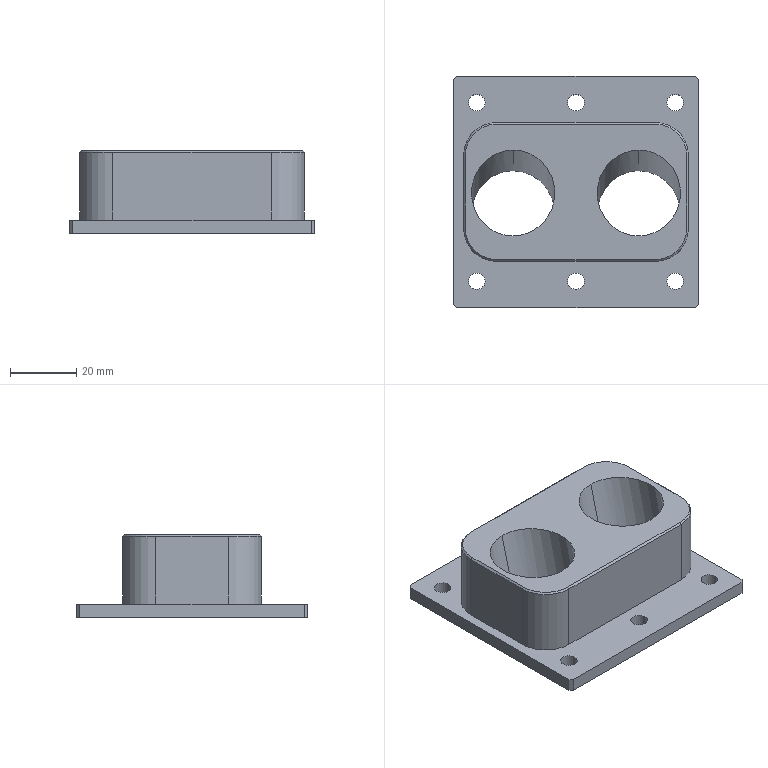Part | SolidWorks | features Chamfer 2, Extrusion 1, ICE 1, MirrorPattern 1, SweepCut 1 | 1 solid | 43 faces | box 74 x 70 x 25 mm | volume 52689 mm3 | cylinder 20 | plane 19 | cone 4 | commonest cylinder face diameters 5 x12 20 x4 25.2 x4
STEP:
#1=CARTESIAN_POINT('',(-19.,-19.566,0.));
#2=VERTEX_POINT('',#1);
#3=CARTESIAN_POINT('',(-19.,6.406,0.));
#4=VERTEX_POINT('',#3);
#5=CARTESIAN_POINT('',(-19.,-19.566,0.));
#6=CARTESIAN_POINT('',(-44.2,-19.566,0.));
#7=CARTESIAN_POINT('',(-44.2,6.406,0.));
#8=CARTESIAN_POINT('',(-19.,6.406,0.));
#9=(BOUNDED_CURVE()B_SPLINE_CURVE(3,(#5,#6,#7,#8),.UNSPECIFIED.,.F.,.F.)B_SPLINE_CURVE_WITH_KNOTS((4,4),(3.142,6.283),.UNSPECIFIED.)CURVE()GEOMETRIC_REPRESENTATION_ITEM()RATIONAL_B_SPLINE_CURVE((1.,0.3333,0.3333,1.))REPRESENTATION_ITEM(''));
#10=EDGE_CURVE('',#2,#4,#9,.T.);
#11=ORIENTED_EDGE('',*,*,#10,.T.);
#12=CARTESIAN_POINT('',(-19.,12.639,25.));
#13=VERTEX_POINT('',#12);
#14=CARTESIAN_POINT('',(-19.,4.636,-7.097));
#15=DIRECTION('',(0.,0.2419,0.9703));
#16=VECTOR('',#15,1000.);
#17=LINE('',#14,#16);
#18=EDGE_CURVE('',#4,#13,#17,.T.);
#19=ORIENTED_EDGE('',*,*,#18,.T.);
#20=CARTESIAN_POINT('',(-19.,-13.333,25.));
#21=VERTEX_POINT('',#20);
#22=CARTESIAN_POINT('',(-19.,12.639,25.));
#23=CARTESIAN_POINT('',(-44.2,12.639,25.));
#24=CARTESIAN_POINT('',(-44.2,-13.333,25.));
#25=CARTESIAN_POINT('',(-19.,-13.333,25.));
#26=(BOUNDED_CURVE()B_SPLINE_CURVE(3,(#22,#23,#24,#25),.UNSPECIFIED.,.F.,.F.)B_SPLINE_CURVE_WITH_KNOTS((4,4),(0.,3.142),.UNSPECIFIED.)CURVE()GEOMETRIC_REPRESENTATION_ITEM()RATIONAL_B_SPLINE_CURVE((1.,0.3333,0.3333,1.))REPRESENTATION_ITEM(''));
#27=EDGE_CURVE('',#13,#21,#26,.T.);
#28=ORIENTED_EDGE('',*,*,#27,.T.);
#29=CARTESIAN_POINT('',(-19.,-19.815,-1.001));
#30=DIRECTION('',(0.,0.2419,0.9703));
#31=VECTOR('',#30,1000.);
#32=LINE('',#29,#31);
#33=EDGE_CURVE('',#2,#21,#32,.T.);
#34=ORIENTED_EDGE('',*,*,#33,.F.);
#35=EDGE_LOOP('',(#11,#19,#28,#34));
#36=FACE_OUTER_BOUND('',#35,.T.);
#37=CARTESIAN_POINT('',(-19.,-7.59,-4.049));
#38=DIRECTION('',(0.,0.2419,0.9703));
#39=DIRECTION('',(0.,-0.9703,0.2419));
#40=AXIS2_PLACEMENT_3D('',#37,#38,#39);
#41=CYLINDRICAL_SURFACE('',#40,12.6);
#42=ADVANCED_FACE('',(#36),#41,.F.);
#43=CARTESIAN_POINT('',(19.,-19.566,0.));
#44=VERTEX_POINT('',#43);
#45=CARTESIAN_POINT('',(19.,6.406,0.));
#46=VERTEX_POINT('',#45);
#47=CARTESIAN_POINT('',(19.,-19.566,0.));
#48=CARTESIAN_POINT('',(-6.2,-19.566,0.));
#49=CARTESIAN_POINT('',(-6.2,6.406,0.));
#50=CARTESIAN_POINT('',(19.,6.406,0.));
#51=(BOUNDED_CURVE()B_SPLINE_CURVE(3,(#47,#48,#49,#50),.UNSPECIFIED.,.F.,.F.)B_SPLINE_CURVE_WITH_KNOTS((4,4),(3.142,6.283),.UNSPECIFIED.)CURVE()GEOMETRIC_REPRESENTATION_ITEM()RATIONAL_B_SPLINE_CURVE((1.,0.3333,0.3333,1.))REPRESENTATION_ITEM(''));
#52=EDGE_CURVE('',#44,#46,#51,.T.);
#53=ORIENTED_EDGE('',*,*,#52,.T.);
#54=CARTESIAN_POINT('',(19.,12.639,25.));
#55=VERTEX_POINT('',#54);
#56=CARTESIAN_POINT('',(19.,4.636,-7.097));
#57=DIRECTION('',(0.,0.2419,0.9703));
#58=VECTOR('',#57,1000.);
#59=LINE('',#56,#58);
#60=EDGE_CURVE('',#46,#55,#59,.T.);
#61=ORIENTED_EDGE('',*,*,#60,.T.);
#62=CARTESIAN_POINT('',(19.,-13.333,25.));
#63=VERTEX_POINT('',#62);
#64=CARTESIAN_POINT('',(19.,12.639,25.));
#65=CARTESIAN_POINT('',(-6.2,12.639,25.));
#66=CARTESIAN_POINT('',(-6.2,-13.333,25.));
#67=CARTESIAN_POINT('',(19.,-13.333,25.));
#68=(BOUNDED_CURVE()B_SPLINE_CURVE(3,(#64,#65,#66,#67),.UNSPECIFIED.,.F.,.F.)B_SPLINE_CURVE_WITH_KNOTS((4,4),(0.,3.142),.UNSPECIFIED.)CURVE()GEOMETRIC_REPRESENTATION_ITEM()RATIONAL_B_SPLINE_CURVE((1.,0.3333,0.3333,1.))REPRESENTATION_ITEM(''));
#69=EDGE_CURVE('',#55,#63,#68,.T.);
#70=ORIENTED_EDGE('',*,*,#69,.T.);
#71=CARTESIAN_POINT('',(19.,-19.815,-1.001));
#72=DIRECTION('',(0.,0.2419,0.9703));
#73=VECTOR('',#72,1000.);
#74=LINE('',#71,#73);
#75=EDGE_CURVE('',#44,#63,#74,.T.);
#76=ORIENTED_EDGE('',*,*,#75,.F.);
#77=EDGE_LOOP('',(#53,#61,#70,#76));
#78=FACE_OUTER_BOUND('',#77,.T.);
#79=CARTESIAN_POINT('',(19.,-7.59,-4.049));
#80=DIRECTION('',(0.,0.2419,0.9703));
#81=DIRECTION('',(0.,-0.9703,0.2419));
#82=AXIS2_PLACEMENT_3D('',#79,#80,#81);
#83=CYLINDRICAL_SURFACE('',#82,12.6);
#84=ADVANCED_FACE('',(#78),#83,.F.);
#85=CARTESIAN_POINT('',(-32.5,-27.,4.));
#86=VERTEX_POINT('',#85);
#87=CARTESIAN_POINT('',(-27.5,-27.,4.));
#88=VERTEX_POINT('',#87);
#89=CARTESIAN_POINT('',(-30.,-27.,4.));
#90=DIRECTION('',(0.,0.,1.));
#91=DIRECTION('',(1.,0.,0.));
#92=AXIS2_PLACEMENT_3D('',#89,#90,#91);
#93=CIRCLE('',#92,2.5);
#94=EDGE_CURVE('',#86,#88,#93,.T.);
#95=ORIENTED_EDGE('',*,*,#94,.T.);
#96=CARTESIAN_POINT('',(-27.5,-27.,0.));
#97=VERTEX_POINT('',#96);
#98=CARTESIAN_POINT('',(-27.5,-27.,4.));
#99=DIRECTION('',(0.,0.,-1.));
#100=VECTOR('',#99,1000.);
#101=LINE('',#98,#100);
#102=EDGE_CURVE('',#88,#97,#101,.T.);
#103=ORIENTED_EDGE('',*,*,#102,.T.);
#104=CARTESIAN_POINT('',(-32.5,-27.,0.));
#105=VERTEX_POINT('',#104);
#106=CARTESIAN_POINT('',(-30.,-27.,0.));
#107=DIRECTION('',(0.,0.,1.));
#108=DIRECTION('',(1.,0.,0.));
#109=AXIS2_PLACEMENT_3D('',#106,#107,#108);
#110=CIRCLE('',#109,2.5);
#111=EDGE_CURVE('',#105,#97,#110,.T.);
#112=ORIENTED_EDGE('',*,*,#111,.F.);
#113=CARTESIAN_POINT('',(-32.5,-27.,4.));
#114=DIRECTION('',(0.,0.,-1.));
#115=VECTOR('',#114,1000.);
#116=LINE('',#113,#115);
#117=EDGE_CURVE('',#86,#105,#116,.T.);
#118=ORIENTED_EDGE('',*,*,#117,.F.);
#119=EDGE_LOOP('',(#95,#103,#112,#118));
#120=FACE_OUTER_BOUND('',#119,.T.);
#121=CARTESIAN_POINT('',(-30.,-27.,4.));
#122=DIRECTION('',(0.,0.,-1.));
#123=DIRECTION('',(-1.,0.,0.));
#124=AXIS2_PLACEMENT_3D('',#121,#122,#123);
#125=CYLINDRICAL_SURFACE('',#124,2.5);
#126=ADVANCED_FACE('',(#120),#125,.F.);
#127=CARTESIAN_POINT('',(-2.5,-27.,4.));
#128=VERTEX_POINT('',#127);
#129=CARTESIAN_POINT('',(2.5,-27.,4.));
#130=VERTEX_POINT('',#129);
#131=CARTESIAN_POINT('',(0.,-27.,4.));
#132=DIRECTION('',(0.,0.,1.));
#133=DIRECTION('',(1.,0.,0.));
#134=AXIS2_PLACEMENT_3D('',#131,#132,#133);
#135=CIRCLE('',#134,2.5);
#136=EDGE_CURVE('',#128,#130,#135,.T.);
#137=ORIENTED_EDGE('',*,*,#136,.T.);
#138=CARTESIAN_POINT('',(2.5,-27.,0.));
#139=VERTEX_POINT('',#138);
#140=CARTESIAN_POINT('',(2.5,-27.,4.));
#141=DIRECTION('',(0.,0.,-1.));
#142=VECTOR('',#141,1000.);
#143=LINE('',#140,#142);
#144=EDGE_CURVE('',#130,#139,#143,.T.);
#145=ORIENTED_EDGE('',*,*,#144,.T.);
#146=CARTESIAN_POINT('',(-2.5,-27.,0.));
#147=VERTEX_POINT('',#146);
#148=CARTESIAN_POINT('',(0.,-27.,0.));
#149=DIRECTION('',(0.,0.,1.));
#150=DIRECTION('',(1.,0.,0.));
#151=AXIS2_PLACEMENT_3D('',#148,#149,#150);
#152=CIRCLE('',#151,2.5);
#153=EDGE_CURVE('',#147,#139,#152,.T.);
#154=ORIENTED_EDGE('',*,*,#153,.F.);
#155=CARTESIAN_POINT('',(-2.5,-27.,4.));
#156=DIRECTION('',(0.,0.,-1.));
#157=VECTOR('',#156,1000.);
#158=LINE('',#155,#157);
#159=EDGE_CURVE('',#128,#147,#158,.T.);
#160=ORIENTED_EDGE('',*,*,#159,.F.);
#161=EDGE_LOOP('',(#137,#145,#154,#160));
#162=FACE_OUTER_BOUND('',#161,.T.);
#163=CARTESIAN_POINT('',(0.,-27.,4.));
#164=DIRECTION('',(0.,0.,-1.));
#165=DIRECTION('',(-1.,0.,0.));
#166=AXIS2_PLACEMENT_3D('',#163,#164,#165);
#167=CYLINDRICAL_SURFACE('',#166,2.5);
#168=ADVANCED_FACE('',(#162),#167,.F.);
#169=CARTESIAN_POINT('',(27.5,-27.,4.));
#170=VERTEX_POINT('',#169);
#171=CARTESIAN_POINT('',(32.5,-27.,4.));
#172=VERTEX_POINT('',#171);
#173=CARTESIAN_POINT('',(30.,-27.,4.));
#174=DIRECTION('',(0.,0.,1.));
#175=DIRECTION('',(1.,0.,0.));
#176=AXIS2_PLACEMENT_3D('',#173,#174,#175);
#177=CIRCLE('',#176,2.5);
#178=EDGE_CURVE('',#170,#172,#177,.T.);
#179=ORIENTED_EDGE('',*,*,#178,.T.);
#180=CARTESIAN_POINT('',(32.5,-27.,0.));
#181=VERTEX_POINT('',#180);
#182=CARTESIAN_POINT('',(32.5,-27.,4.));
#183=DIRECTION('',(0.,0.,-1.));
#184=VECTOR('',#183,1000.);
#185=LINE('',#182,#184);
#186=EDGE_CURVE('',#172,#181,#185,.T.);
#187=ORIENTED_EDGE('',*,*,#186,.T.);
#188=CARTESIAN_POINT('',(27.5,-27.,0.));
#189=VERTEX_POINT('',#188);
#190=CARTESIAN_POINT('',(30.,-27.,0.));
#191=DIRECTION('',(0.,0.,1.));
#192=DIRECTION('',(1.,0.,0.));
#193=AXIS2_PLACEMENT_3D('',#190,#191,#192);
#194=CIRCLE('',#193,2.5);
#195=EDGE_CURVE('',#189,#181,#194,.T.);
#196=ORIENTED_EDGE('',*,*,#195,.F.);
#197=CARTESIAN_POINT('',(27.5,-27.,4.));
#198=DIRECTION('',(0.,0.,-1.));
#199=VECTOR('',#198,1000.);
#200=LINE('',#197,#199);
#201=EDGE_CURVE('',#170,#189,#200,.T.);
#202=ORIENTED_EDGE('',*,*,#201,.F.);
#203=EDGE_LOOP('',(#179,#187,#196,#202));
#204=FACE_OUTER_BOUND('',#203,.T.);
#205=CARTESIAN_POINT('',(30.,-27.,4.));
#206=DIRECTION('',(0.,0.,-1.));
#207=DIRECTION('',(-1.,0.,0.));
#208=AXIS2_PLACEMENT_3D('',#205,#206,#207);
#209=CYLINDRICAL_SURFACE('',#208,2.5);
#210=ADVANCED_FACE('',(#204),#209,.F.);
#211=CARTESIAN_POINT('',(27.5,27.,4.));
#212=VERTEX_POINT('',#211);
#213=CARTESIAN_POINT('',(32.5,27.,4.));
#214=VERTEX_POINT('',#213);
#215=CARTESIAN_POINT('',(30.,27.,4.));
#216=DIRECTION('',(0.,0.,1.));
#217=DIRECTION('',(1.,0.,0.));
#218=AXIS2_PLACEMENT_3D('',#215,#216,#217);
#219=CIRCLE('',#218,2.5);
#220=EDGE_CURVE('',#212,#214,#219,.T.);
#221=ORIENTED_EDGE('',*,*,#220,.T.);
#222=CARTESIAN_POINT('',(32.5,27.,0.));
#223=VERTEX_POINT('',#222);
#224=CARTESIAN_POINT('',(32.5,27.,4.));
#225=DIRECTION('',(0.,0.,-1.));
#226=VECTOR('',#225,1000.);
#227=LINE('',#224,#226);
#228=EDGE_CURVE('',#214,#223,#227,.T.);
#229=ORIENTED_EDGE('',*,*,#228,.T.);
#230=CARTESIAN_POINT('',(27.5,27.,0.));
#231=VERTEX_POINT('',#230);
#232=CARTESIAN_POINT('',(30.,27.,0.));
#233=DIRECTION('',(0.,0.,1.));
#234=DIRECTION('',(1.,0.,0.));
#235=AXIS2_PLACEMENT_3D('',#232,#233,#234);
#236=CIRCLE('',#235,2.5);
#237=EDGE_CURVE('',#231,#223,#236,.T.);
#238=ORIENTED_EDGE('',*,*,#237,.F.);
#239=CARTESIAN_POINT('',(27.5,27.,4.));
#240=DIRECTION('',(0.,0.,-1.));
#241=VECTOR('',#240,1000.);
#242=LINE('',#239,#241);
#243=EDGE_CURVE('',#212,#231,#242,.T.);
#244=ORIENTED_EDGE('',*,*,#243,.F.);
#245=EDGE_LOOP('',(#221,#229,#238,#244));
#246=FACE_OUTER_BOUND('',#245,.T.);
#247=CARTESIAN_POINT('',(30.,27.,4.));
#248=DIRECTION('',(0.,0.,-1.));
#249=DIRECTION('',(-1.,0.,0.));
#250=AXIS2_PLACEMENT_3D('',#247,#248,#249);
#251=CYLINDRICAL_SURFACE('',#250,2.5);
#252=ADVANCED_FACE('',(#246),#251,.F.);
#253=CARTESIAN_POINT('',(-2.5,27.,4.));
#254=VERTEX_POINT('',#253);
#255=CARTESIAN_POINT('',(2.5,27.,4.));
#256=VERTEX_POINT('',#255);
#257=CARTESIAN_POINT('',(0.,27.,4.));
#258=DIRECTION('',(0.,0.,1.));
#259=DIRECTION('',(1.,0.,0.));
#260=AXIS2_PLACEMENT_3D('',#257,#258,#259);
#261=CIRCLE('',#260,2.5);
#262=EDGE_CURVE('',#254,#256,#261,.T.);
#263=ORIENTED_EDGE('',*,*,#262,.T.);
#264=CARTESIAN_POINT('',(2.5,27.,0.));
#265=VERTEX_POINT('',#264);
#266=CARTESIAN_POINT('',(2.5,27.,4.));
#267=DIRECTION('',(0.,0.,-1.));
#268=VECTOR('',#267,1000.);
#269=LINE('',#266,#268);
#270=EDGE_CURVE('',#256,#265,#269,.T.);
#271=ORIENTED_EDGE('',*,*,#270,.T.);
#272=CARTESIAN_POINT('',(-2.5,27.,0.));
#273=VERTEX_POINT('',#272);
#274=CARTESIAN_POINT('',(0.,27.,0.));
#275=DIRECTION('',(0.,0.,1.));
#276=DIRECTION('',(1.,0.,0.));
#277=AXIS2_PLACEMENT_3D('',#274,#275,#276);
#278=CIRCLE('',#277,2.5);
#279=EDGE_CURVE('',#273,#265,#278,.T.);
#280=ORIENTED_EDGE('',*,*,#279,.F.);
#281=CARTESIAN_POINT('',(-2.5,27.,4.));
#282=DIRECTION('',(0.,0.,-1.));
#283=VECTOR('',#282,1000.);
#284=LINE('',#281,#283);
#285=EDGE_CURVE('',#254,#273,#284,.T.);
#286=ORIENTED_EDGE('',*,*,#285,.F.);
#287=EDGE_LOOP('',(#263,#271,#280,#286));
#288=FACE_OUTER_BOUND('',#287,.T.);
#289=CARTESIAN_POINT('',(0.,27.,4.));
#290=DIRECTION('',(0.,0.,-1.));
#291=DIRECTION('',(-1.,0.,0.));
#292=AXIS2_PLACEMENT_3D('',#289,#290,#291);
#293=CYLINDRICAL_SURFACE('',#292,2.5);
#294=ADVANCED_FACE('',(#288),#293,.F.);
#295=CARTESIAN_POINT('',(-32.5,27.,4.));
#296=VERTEX_POINT('',#295);
#297=CARTESIAN_POINT('',(-27.5,27.,4.));
#298=VERTEX_POINT('',#297);
#299=CARTESIAN_POINT('',(-30.,27.,4.));
#300=DIRECTION('',(0.,0.,1.));
#301=DIRECTION('',(1.,0.,0.));
#302=AXIS2_PLACEMENT_3D('',#299,#300,#301);
#303=CIRCLE('',#302,2.5);
#304=EDGE_CURVE('',#296,#298,#303,.T.);
#305=ORIENTED_EDGE('',*,*,#304,.T.);
#306=CARTESIAN_POINT('',(-27.5,27.,0.));
#307=VERTEX_POINT('',#306);
#308=CARTESIAN_POINT('',(-27.5,27.,4.));
#309=DIRECTION('',(0.,0.,-1.));
#310=VECTOR('',#309,1000.);
#311=LINE('',#308,#310);
#312=EDGE_CURVE('',#298,#307,#311,.T.);
#313=ORIENTED_EDGE('',*,*,#312,.T.);
#314=CARTESIAN_POINT('',(-32.5,27.,0.));
#315=VERTEX_POINT('',#314);
#316=CARTESIAN_POINT('',(-30.,27.,0.));
#317=DIRECTION('',(0.,0.,1.));
#318=DIRECTION('',(1.,0.,0.));
#319=AXIS2_PLACEMENT_3D('',#316,#317,#318);
#320=CIRCLE('',#319,2.5);
#321=EDGE_CURVE('',#315,#307,#320,.T.);
#322=ORIENTED_EDGE('',*,*,#321,.F.);
#323=CARTESIAN_POINT('',(-32.5,27.,4.));
#324=DIRECTION('',(0.,0.,-1.));
#325=VECTOR('',#324,1000.);
#326=LINE('',#323,#325);
#327=EDGE_CURVE('',#296,#315,#326,.T.);
#328=ORIENTED_EDGE('',*,*,#327,.F.);
#329=EDGE_LOOP('',(#305,#313,#322,#328));
#330=FACE_OUTER_BOUND('',#329,.T.);
#331=CARTESIAN_POINT('',(-30.,27.,4.));
#332=DIRECTION('',(0.,0.,-1.));
#333=DIRECTION('',(-1.,0.,0.));
#334=AXIS2_PLACEMENT_3D('',#331,#332,#333);
#335=CYLINDRICAL_SURFACE('',#334,2.5);
#336=ADVANCED_FACE('',(#330),#335,.F.);
#337=ORIENTED_EDGE('',*,*,#94,.F.);
#338=CARTESIAN_POINT('',(-30.,-27.,4.));
#339=DIRECTION('',(0.,0.,1.));
#340=DIRECTION('',(1.,0.,0.));
#341=AXIS2_PLACEMENT_3D('',#338,#339,#340);
#342=CIRCLE('',#341,2.5);
#343=EDGE_CURVE('',#88,#86,#342,.T.);
#344=ORIENTED_EDGE('',*,*,#343,.F.);
#345=EDGE_LOOP('',(#337,#344));
#346=FACE_BOUND('',#345,.T.);
#347=ORIENTED_EDGE('',*,*,#136,.F.);
#348=CARTESIAN_POINT('',(0.,-27.,4.));
#349=DIRECTION('',(0.,0.,1.));
#350=DIRECTION('',(1.,0.,0.));
#351=AXIS2_PLACEMENT_3D('',#348,#349,#350);
#352=CIRCLE('',#351,2.5);
#353=EDGE_CURVE('',#130,#128,#352,.T.);
#354=ORIENTED_EDGE('',*,*,#353,.F.);
#355=EDGE_LOOP('',(#347,#354));
#356=FACE_BOUND('',#355,.T.);
#357=ORIENTED_EDGE('',*,*,#178,.F.);
#358=CARTESIAN_POINT('',(30.,-27.,4.));
#359=DIRECTION('',(0.,0.,1.));
#360=DIRECTION('',(1.,0.,0.));
#361=AXIS2_PLACEMENT_3D('',#358,#359,#360);
#362=CIRCLE('',#361,2.5);
#363=EDGE_CURVE('',#172,#170,#362,.T.);
#364=ORIENTED_EDGE('',*,*,#363,.F.);
#365=EDGE_LOOP('',(#357,#364));
#366=FACE_BOUND('',#365,.T.);
#367=ORIENTED_EDGE('',*,*,#220,.F.);
#368=CARTESIAN_POINT('',(30.,27.,4.));
#369=DIRECTION('',(0.,0.,1.));
#370=DIRECTION('',(1.,0.,0.));
#371=AXIS2_PLACEMENT_3D('',#368,#369,#370);
#372=CIRCLE('',#371,2.5);
#373=EDGE_CURVE('',#214,#212,#372,.T.);
#374=ORIENTED_EDGE('',*,*,#373,.F.);
#375=EDGE_LOOP('',(#367,#374));
#376=FACE_BOUND('',#375,.T.);
#377=ORIENTED_EDGE('',*,*,#262,.F.);
#378=CARTESIAN_POINT('',(0.,27.,4.));
#379=DIRECTION('',(0.,0.,1.));
#380=DIRECTION('',(1.,0.,0.));
#381=AXIS2_PLACEMENT_3D('',#378,#379,#380);
#382=CIRCLE('',#381,2.5);
#383=EDGE_CURVE('',#256,#254,#382,.T.);
#384=ORIENTED_EDGE('',*,*,#383,.F.);
#385=EDGE_LOOP('',(#377,#384));
#386=FACE_BOUND('',#385,.T.);
#387=ORIENTED_EDGE('',*,*,#304,.F.);
#388=CARTESIAN_POINT('',(-30.,27.,4.));
#389=DIRECTION('',(0.,0.,1.));
#390=DIRECTION('',(1.,0.,0.));
#391=AXIS2_PLACEMENT_3D('',#388,#389,#390);
#392=CIRCLE('',#391,2.5);
#393=EDGE_CURVE('',#298,#296,#392,.T.);
#394=ORIENTED_EDGE('',*,*,#393,.F.);
#395=EDGE_LOOP('',(#387,#394));
#396=FACE_BOUND('',#395,.T.);
#397=CARTESIAN_POINT('',(-36.,-35.,4.));
#398=VERTEX_POINT('',#397);
#399=CARTESIAN_POINT('',(36.,-35.,4.));
#400=VERTEX_POINT('',#399);
#401=CARTESIAN_POINT('',(0.,-35.,4.));
#402=DIRECTION('',(1.,0.,0.));
#403=VECTOR('',#402,1000.);
#404=LINE('',#401,#403);
#405=EDGE_CURVE('',#398,#400,#404,.T.);
#406=ORIENTED_EDGE('',*,*,#405,.T.);
#407=CARTESIAN_POINT('',(37.,-34.,4.));
#408=VERTEX_POINT('',#407);
#409=CARTESIAN_POINT('',(35.5,-35.5,4.));
#410=DIRECTION('',(0.7071,0.7071,0.));
#411=VECTOR('',#410,1000.);
#412=LINE('',#409,#411);
#413=EDGE_CURVE('',#400,#408,#412,.T.);
#414=ORIENTED_EDGE('',*,*,#413,.T.);
#415=CARTESIAN_POINT('',(37.,34.,4.));
#416=VERTEX_POINT('',#415);
#417=CARTESIAN_POINT('',(37.,0.,4.));
#418=DIRECTION('',(0.,1.,0.));
#419=VECTOR('',#418,1000.);
#420=LINE('',#417,#419);
#421=EDGE_CURVE('',#408,#416,#420,.T.);
#422=ORIENTED_EDGE('',*,*,#421,.T.);
#423=CARTESIAN_POINT('',(36.,35.,4.));
#424=VERTEX_POINT('',#423);
#425=CARTESIAN_POINT('',(35.5,35.5,4.));
#426=DIRECTION('',(-0.7071,0.7071,0.));
#427=VECTOR('',#426,1000.);
#428=LINE('',#425,#427);
#429=EDGE_CURVE('',#416,#424,#428,.T.);
#430=ORIENTED_EDGE('',*,*,#429,.T.);
#431=CARTESIAN_POINT('',(-36.,35.,4.));
#432=VERTEX_POINT('',#431);
#433=CARTESIAN_POINT('',(0.,35.,4.));
#434=DIRECTION('',(1.,0.,0.));
#435=VECTOR('',#434,1000.);
#436=LINE('',#433,#435);
#437=EDGE_CURVE('',#432,#424,#436,.T.);
#438=ORIENTED_EDGE('',*,*,#437,.F.);
#439=CARTESIAN_POINT('',(-37.,34.,4.));
#440=VERTEX_POINT('',#439);
#441=CARTESIAN_POINT('',(-35.5,35.5,4.));
#442=DIRECTION('',(-0.7071,-0.7071,0.));
#443=VECTOR('',#442,1000.);
#444=LINE('',#441,#443);
#445=EDGE_CURVE('',#432,#440,#444,.T.);
#446=ORIENTED_EDGE('',*,*,#445,.T.);
#447=CARTESIAN_POINT('',(-37.,-34.,4.));
#448=VERTEX_POINT('',#447);
#449=CARTESIAN_POINT('',(-37.,0.,4.));
#450=DIRECTION('',(0.,1.,0.));
#451=VECTOR('',#450,1000.);
#452=LINE('',#449,#451);
#453=EDGE_CURVE('',#448,#440,#452,.T.);
#454=ORIENTED_EDGE('',*,*,#453,.F.);
#455=CARTESIAN_POINT('',(-35.5,-35.5,4.));
#456=DIRECTION('',(0.7071,-0.7071,0.));
#457=VECTOR('',#456,1000.);
#458=LINE('',#455,#457);
#459=EDGE_CURVE('',#448,#398,#458,.T.);
#460=ORIENTED_EDGE('',*,*,#459,.T.);
#461=EDGE_LOOP('',(#406,#414,#422,#430,#438,#446,#454,#460));
#462=FACE_OUTER_BOUND('',#461,.T.);
#463=CARTESIAN_POINT('',(24.,21.,4.));
#464=VERTEX_POINT('',#463);
#465=CARTESIAN_POINT('',(-24.,21.,4.));
#466=VERTEX_POINT('',#465);
#467=CARTESIAN_POINT('',(-24.,21.,4.));
#468=DIRECTION('',(-1.,0.,0.));
#469=VECTOR('',#468,1000.);
#470=LINE('',#467,#469);
#471=EDGE_CURVE('',#464,#466,#470,.T.);
#472=ORIENTED_EDGE('',*,*,#471,.F.);
#473=CARTESIAN_POINT('',(34.,11.,4.));
#474=VERTEX_POINT('',#473);
#475=CARTESIAN_POINT('',(24.,11.,4.));
#476=DIRECTION('',(0.,0.,1.));
#477=DIRECTION('',(-1.,0.,0.));
#478=AXIS2_PLACEMENT_3D('',#475,#476,#477);
#479=CIRCLE('',#478,10.);
#480=EDGE_CURVE('',#474,#464,#479,.T.);
#481=ORIENTED_EDGE('',*,*,#480,.F.);
#482=CARTESIAN_POINT('',(34.,-11.,4.));
#483=VERTEX_POINT('',#482);
#484=CARTESIAN_POINT('',(34.,-11.,4.));
#485=DIRECTION('',(0.,1.,0.));
#486=VECTOR('',#485,1000.);
#487=LINE('',#484,#486);
#488=EDGE_CURVE('',#483,#474,#487,.T.);
#489=ORIENTED_EDGE('',*,*,#488,.F.);
#490=CARTESIAN_POINT('',(24.,-21.,4.));
#491=VERTEX_POINT('',#490);
#492=CARTESIAN_POINT('',(24.,-11.,4.));
#493=DIRECTION('',(0.,0.,1.));
#494=DIRECTION('',(-1.,0.,0.));
#495=AXIS2_PLACEMENT_3D('',#492,#493,#494);
#496=CIRCLE('',#495,10.);
#497=EDGE_CURVE('',#491,#483,#496,.T.);
#498=ORIENTED_EDGE('',*,*,#497,.F.);
#499=CARTESIAN_POINT('',(-24.,-21.,4.));
#500=VERTEX_POINT('',#499);
#501=CARTESIAN_POINT('',(-24.,-21.,4.));
#502=DIRECTION('',(1.,0.,0.));
#503=VECTOR('',#502,1000.);
#504=LINE('',#501,#503);
#505=EDGE_CURVE('',#500,#491,#504,.T.);
#506=ORIENTED_EDGE('',*,*,#505,.F.);
#507=CARTESIAN_POINT('',(-34.,-11.,4.));
#508=VERTEX_POINT('',#507);
#509=CARTESIAN_POINT('',(-24.,-11.,4.));
#510=DIRECTION('',(0.,0.,1.));
#511=DIRECTION('',(-1.,0.,0.));
#512=AXIS2_PLACEMENT_3D('',#509,#510,#511);
#513=CIRCLE('',#512,10.);
#514=EDGE_CURVE('',#508,#500,#513,.T.);
#515=ORIENTED_EDGE('',*,*,#514,.F.);
#516=CARTESIAN_POINT('',(-34.,11.,4.));
#517=VERTEX_POINT('',#516);
#518=CARTESIAN_POINT('',(-34.,-11.,4.));
#519=DIRECTION('',(0.,-1.,0.));
#520=VECTOR('',#519,1000.);
#521=LINE('',#518,#520);
#522=EDGE_CURVE('',#517,#508,#521,.T.);
#523=ORIENTED_EDGE('',*,*,#522,.F.);
#524=CARTESIAN_POINT('',(-24.,11.,4.));
#525=DIRECTION('',(0.,0.,1.));
#526=DIRECTION('',(-1.,0.,0.));
#527=AXIS2_PLACEMENT_3D('',#524,#525,#526);
#528=CIRCLE('',#527,10.);
#529=EDGE_CURVE('',#466,#517,#528,.T.);
#530=ORIENTED_EDGE('',*,*,#529,.F.);
#531=EDGE_LOOP('',(#472,#481,#489,#498,#506,#515,#523,#530));
#532=FACE_BOUND('',#531,.T.);
#533=CARTESIAN_POINT('',(0.,0.,4.));
#534=DIRECTION('',(0.,0.,1.));
#535=DIRECTION('',(1.,0.,0.));
#536=AXIS2_PLACEMENT_3D('',#533,#534,#535);
#537=PLANE('',#536);
#538=ADVANCED_FACE('',(#346,#356,#366,#376,#386,#396,#462,#532),#537,.T.);
#539=CARTESIAN_POINT('',(-36.,-35.,0.));
#540=VERTEX_POINT('',#539);
#541=CARTESIAN_POINT('',(36.,-35.,0.));
#542=VERTEX_POINT('',#541);
#543=CARTESIAN_POINT('',(0.,-35.,0.));
#544=DIRECTION('',(1.,0.,0.));
#545=VECTOR('',#544,1000.);
#546=LINE('',#543,#545);
#547=EDGE_CURVE('',#540,#542,#546,.T.);
#548=ORIENTED_EDGE('',*,*,#547,.T.);
#549=CARTESIAN_POINT('',(36.,-35.,4.));
#550=DIRECTION('',(0.,0.,1.));
#551=VECTOR('',#550,1000.);
#552=LINE('',#549,#551);
#553=EDGE_CURVE('',#542,#400,#552,.T.);
#554=ORIENTED_EDGE('',*,*,#553,.T.);
#555=ORIENTED_EDGE('',*,*,#405,.F.);
#556=CARTESIAN_POINT('',(-36.,-35.,0.));
#557=DIRECTION('',(0.,0.,-1.));
#558=VECTOR('',#557,1000.);
#559=LINE('',#556,#558);
#560=EDGE_CURVE('',#398,#540,#559,.T.);
#561=ORIENTED_EDGE('',*,*,#560,.T.);
#562=EDGE_LOOP('',(#548,#554,#555,#561));
#563=FACE_OUTER_BOUND('',#562,.T.);
#564=CARTESIAN_POINT('',(0.,-35.,4.));
#565=DIRECTION('',(0.,1.,0.));
#566=DIRECTION('',(0.,0.,1.));
#567=AXIS2_PLACEMENT_3D('',#564,#565,#566);
#568=PLANE('',#567);
#569=ADVANCED_FACE('',(#563),#568,.F.);
#570=ORIENTED_EDGE('',*,*,#421,.F.);
#571=CARTESIAN_POINT('',(37.,-34.,0.));
#572=VERTEX_POINT('',#571);
#573=CARTESIAN_POINT('',(37.,-34.,4.));
#574=DIRECTION('',(0.,0.,-1.));
#575=VECTOR('',#574,1000.);
#576=LINE('',#573,#575);
#577=EDGE_CURVE('',#408,#572,#576,.T.);
#578=ORIENTED_EDGE('',*,*,#577,.T.);
#579=CARTESIAN_POINT('',(37.,34.,0.));
#580=VERTEX_POINT('',#579);
#581=CARTESIAN_POINT('',(37.,0.,0.));
#582=DIRECTION('',(0.,1.,0.));
#583=VECTOR('',#582,1000.);
#584=LINE('',#581,#583);
#585=EDGE_CURVE('',#572,#580,#584,.T.);
#586=ORIENTED_EDGE('',*,*,#585,.T.);
#587=CARTESIAN_POINT('',(37.,34.,4.));
#588=DIRECTION('',(0.,0.,1.));
#589=VECTOR('',#588,1000.);
#590=LINE('',#587,#589);
#591=EDGE_CURVE('',#580,#416,#590,.T.);
#592=ORIENTED_EDGE('',*,*,#591,.T.);
#593=EDGE_LOOP('',(#570,#578,#586,#592));
#594=FACE_OUTER_BOUND('',#593,.T.);
#595=CARTESIAN_POINT('',(37.,0.,4.));
#596=DIRECTION('',(-1.,0.,0.));
#597=DIRECTION('',(0.,0.,1.));
#598=AXIS2_PLACEMENT_3D('',#595,#596,#597);
#599=PLANE('',#598);
#600=ADVANCED_FACE('',(#594),#599,.F.);
#601=ORIENTED_EDGE('',*,*,#437,.T.);
#602=CARTESIAN_POINT('',(36.,35.,0.));
#603=VERTEX_POINT('',#602);
#604=CARTESIAN_POINT('',(36.,35.,0.));
#605=DIRECTION('',(0.,0.,-1.));
#606=VECTOR('',#605,1000.);
#607=LINE('',#604,#606);
#608=EDGE_CURVE('',#424,#603,#607,.T.);
#609=ORIENTED_EDGE('',*,*,#608,.T.);
#610=CARTESIAN_POINT('',(-36.,35.,0.));
#611=VERTEX_POINT('',#610);
#612=CARTESIAN_POINT('',(0.,35.,0.));
#613=DIRECTION('',(1.,0.,0.));
#614=VECTOR('',#613,1000.);
#615=LINE('',#612,#614);
#616=EDGE_CURVE('',#611,#603,#615,.T.);
#617=ORIENTED_EDGE('',*,*,#616,.F.);
#618=CARTESIAN_POINT('',(-36.,35.,4.));
#619=DIRECTION('',(0.,0.,1.));
#620=VECTOR('',#619,1000.);
#621=LINE('',#618,#620);
#622=EDGE_CURVE('',#611,#432,#621,.T.);
#623=ORIENTED_EDGE('',*,*,#622,.T.);
#624=EDGE_LOOP('',(#601,#609,#617,#623));
#625=FACE_OUTER_BOUND('',#624,.T.);
#626=CARTESIAN_POINT('',(0.,35.,4.));
#627=DIRECTION('',(0.,1.,0.));
#628=DIRECTION('',(0.,0.,1.));
#629=AXIS2_PLACEMENT_3D('',#626,#627,#628);
#630=PLANE('',#629);
#631=ADVANCED_FACE('',(#625),#630,.T.);
#632=ORIENTED_EDGE('',*,*,#312,.F.);
#633=ORIENTED_EDGE('',*,*,#393,.T.);
#634=ORIENTED_EDGE('',*,*,#327,.T.);
#635=CARTESIAN_POINT('',(-30.,27.,0.));
#636=DIRECTION('',(0.,0.,1.));
#637=DIRECTION('',(1.,0.,0.));
#638=AXIS2_PLACEMENT_3D('',#635,#636,#637);
#639=CIRCLE('',#638,2.5);
#640=EDGE_CURVE('',#307,#315,#639,.T.);
#641=ORIENTED_EDGE('',*,*,#640,.F.);
#642=EDGE_LOOP('',(#632,#633,#634,#641));
#643=FACE_OUTER_BOUND('',#642,.T.);
#644=CARTESIAN_POINT('',(-30.,27.,4.));
#645=DIRECTION('',(0.,0.,-1.));
#646=DIRECTION('',(-1.,0.,0.));
#647=AXIS2_PLACEMENT_3D('',#644,#645,#646);
#648=CYLINDRICAL_SURFACE('',#647,2.5);
#649=ADVANCED_FACE('',(#643),#648,.F.);
#650=ORIENTED_EDGE('',*,*,#270,.F.);
#651=ORIENTED_EDGE('',*,*,#383,.T.);
#652=ORIENTED_EDGE('',*,*,#285,.T.);
#653=CARTESIAN_POINT('',(0.,27.,0.));
#654=DIRECTION('',(0.,0.,1.));
#655=DIRECTION('',(1.,0.,0.));
#656=AXIS2_PLACEMENT_3D('',#653,#654,#655);
#657=CIRCLE('',#656,2.5);
#658=EDGE_CURVE('',#265,#273,#657,.T.);
#659=ORIENTED_EDGE('',*,*,#658,.F.);
#660=EDGE_LOOP('',(#650,#651,#652,#659));
#661=FACE_OUTER_BOUND('',#660,.T.);
#662=CARTESIAN_POINT('',(0.,27.,4.));
#663=DIRECTION('',(0.,0.,-1.));
#664=DIRECTION('',(-1.,0.,0.));
#665=AXIS2_PLACEMENT_3D('',#662,#663,#664);
#666=CYLINDRICAL_SURFACE('',#665,2.5);
#667=ADVANCED_FACE('',(#661),#666,.F.);
#668=ORIENTED_EDGE('',*,*,#228,.F.);
#669=ORIENTED_EDGE('',*,*,#373,.T.);
#670=ORIENTED_EDGE('',*,*,#243,.T.);
#671=CARTESIAN_POINT('',(30.,27.,0.));
#672=DIRECTION('',(0.,0.,1.));
#673=DIRECTION('',(1.,0.,0.));
#674=AXIS2_PLACEMENT_3D('',#671,#672,#673);
#675=CIRCLE('',#674,2.5);
#676=EDGE_CURVE('',#223,#231,#675,.T.);
#677=ORIENTED_EDGE('',*,*,#676,.F.);
#678=EDGE_LOOP('',(#668,#669,#670,#677));
#679=FACE_OUTER_BOUND('',#678,.T.);
#680=CARTESIAN_POINT('',(30.,27.,4.));
#681=DIRECTION('',(0.,0.,-1.));
#682=DIRECTION('',(-1.,0.,0.));
#683=AXIS2_PLACEMENT_3D('',#680,#681,#682);
#684=CYLINDRICAL_SURFACE('',#683,2.5);
#685=ADVANCED_FACE('',(#679),#684,.F.);
#686=ORIENTED_EDGE('',*,*,#186,.F.);
#687=ORIENTED_EDGE('',*,*,#363,.T.);
#688=ORIENTED_EDGE('',*,*,#201,.T.);
#689=CARTESIAN_POINT('',(30.,-27.,0.));
#690=DIRECTION('',(0.,0.,1.));
#691=DIRECTION('',(1.,0.,0.));
#692=AXIS2_PLACEMENT_3D('',#689,#690,#691);
#693=CIRCLE('',#692,2.5);
#694=EDGE_CURVE('',#181,#189,#693,.T.);
#695=ORIENTED_EDGE('',*,*,#694,.F.);
#696=EDGE_LOOP('',(#686,#687,#688,#695));
#697=FACE_OUTER_BOUND('',#696,.T.);
#698=CARTESIAN_POINT('',(30.,-27.,4.));
#699=DIRECTION('',(0.,0.,-1.));
#700=DIRECTION('',(-1.,0.,0.));
#701=AXIS2_PLACEMENT_3D('',#698,#699,#700);
#702=CYLINDRICAL_SURFACE('',#701,2.5);
#703=ADVANCED_FACE('',(#697),#702,.F.);
#704=ORIENTED_EDGE('',*,*,#144,.F.);
#705=ORIENTED_EDGE('',*,*,#353,.T.);
#706=ORIENTED_EDGE('',*,*,#159,.T.);
#707=CARTESIAN_POINT('',(0.,-27.,0.));
#708=DIRECTION('',(0.,0.,1.));
#709=DIRECTION('',(1.,0.,0.));
#710=AXIS2_PLACEMENT_3D('',#707,#708,#709);
#711=CIRCLE('',#710,2.5);
#712=EDGE_CURVE('',#139,#147,#711,.T.);
#713=ORIENTED_EDGE('',*,*,#712,.F.);
#714=EDGE_LOOP('',(#704,#705,#706,#713));
#715=FACE_OUTER_BOUND('',#714,.T.);
#716=CARTESIAN_POINT('',(0.,-27.,4.));
#717=DIRECTION('',(0.,0.,-1.));
#718=DIRECTION('',(-1.,0.,0.));
#719=AXIS2_PLACEMENT_3D('',#716,#717,#718);
#720=CYLINDRICAL_SURFACE('',#719,2.5);
#721=ADVANCED_FACE('',(#715),#720,.F.);
#722=ORIENTED_EDGE('',*,*,#102,.F.);
#723=ORIENTED_EDGE('',*,*,#343,.T.);
#724=ORIENTED_EDGE('',*,*,#117,.T.);
#725=CARTESIAN_POINT('',(-30.,-27.,0.));
#726=DIRECTION('',(0.,0.,1.));
#727=DIRECTION('',(1.,0.,0.));
#728=AXIS2_PLACEMENT_3D('',#725,#726,#727);
#729=CIRCLE('',#728,2.5);
#730=EDGE_CURVE('',#97,#105,#729,.T.);
#731=ORIENTED_EDGE('',*,*,#730,.F.);
#732=EDGE_LOOP('',(#722,#723,#724,#731));
#733=FACE_OUTER_BOUND('',#732,.T.);
#734=CARTESIAN_POINT('',(-30.,-27.,4.));
#735=DIRECTION('',(0.,0.,-1.));
#736=DIRECTION('',(-1.,0.,0.));
#737=AXIS2_PLACEMENT_3D('',#734,#735,#736);
#738=CYLINDRICAL_SURFACE('',#737,2.5);
#739=ADVANCED_FACE('',(#733),#738,.F.);
#740=CARTESIAN_POINT('',(-37.,-34.,0.));
#741=VERTEX_POINT('',#740);
#742=CARTESIAN_POINT('',(-37.,34.,0.));
#743=VERTEX_POINT('',#742);
#744=CARTESIAN_POINT('',(-37.,0.,0.));
#745=DIRECTION('',(0.,1.,0.));
#746=VECTOR('',#745,1000.);
#747=LINE('',#744,#746);
#748=EDGE_CURVE('',#741,#743,#747,.T.);
#749=ORIENTED_EDGE('',*,*,#748,.F.);
#750=CARTESIAN_POINT('',(-37.,-34.,4.));
#751=DIRECTION('',(0.,0.,1.));
#752=VECTOR('',#751,1000.);
#753=LINE('',#750,#752);
#754=EDGE_CURVE('',#741,#448,#753,.T.);
#755=ORIENTED_EDGE('',*,*,#754,.T.);
#756=ORIENTED_EDGE('',*,*,#453,.T.);
#757=CARTESIAN_POINT('',(-37.,34.,4.));
#758=DIRECTION('',(0.,0.,-1.));
#759=VECTOR('',#758,1000.);
#760=LINE('',#757,#759);
#761=EDGE_CURVE('',#440,#743,#760,.T.);
#762=ORIENTED_EDGE('',*,*,#761,.T.);
#763=EDGE_LOOP('',(#749,#755,#756,#762));
#764=FACE_OUTER_BOUND('',#763,.T.);
#765=CARTESIAN_POINT('',(-37.,0.,4.));
#766=DIRECTION('',(-1.,0.,0.));
#767=DIRECTION('',(0.,0.,1.));
#768=AXIS2_PLACEMENT_3D('',#765,#766,#767);
#769=PLANE('',#768);
#770=ADVANCED_FACE('',(#764),#769,.T.);
#771=ORIENTED_EDGE('',*,*,#10,.F.);
#772=CARTESIAN_POINT('',(-19.,6.406,0.));
#773=CARTESIAN_POINT('',(6.2,6.406,0.));
#774=CARTESIAN_POINT('',(6.2,-19.566,0.));
#775=CARTESIAN_POINT('',(-19.,-19.566,0.));
#776=(BOUNDED_CURVE()B_SPLINE_CURVE(3,(#772,#773,#774,#775),.UNSPECIFIED.,.F.,.F.)B_SPLINE_CURVE_WITH_KNOTS((4,4),(0.,3.142),.UNSPECIFIED.)CURVE()GEOMETRIC_REPRESENTATION_ITEM()RATIONAL_B_SPLINE_CURVE((1.,0.3333,0.3333,1.))REPRESENTATION_ITEM(''));
#777=EDGE_CURVE('',#4,#2,#776,.T.);
#778=ORIENTED_EDGE('',*,*,#777,.F.);
#779=EDGE_LOOP('',(#771,#778));
#780=FACE_BOUND('',#779,.T.);
#781=ORIENTED_EDGE('',*,*,#52,.F.);
#782=CARTESIAN_POINT('',(19.,6.406,0.));
#783=CARTESIAN_POINT('',(44.2,6.406,0.));
#784=CARTESIAN_POINT('',(44.2,-19.566,0.));
#785=CARTESIAN_POINT('',(19.,-19.566,0.));
#786=(BOUNDED_CURVE()B_SPLINE_CURVE(3,(#782,#783,#784,#785),.UNSPECIFIED.,.F.,.F.)B_SPLINE_CURVE_WITH_KNOTS((4,4),(0.,3.142),.UNSPECIFIED.)CURVE()GEOMETRIC_REPRESENTATION_ITEM()RATIONAL_B_SPLINE_CURVE((1.,0.3333,0.3333,1.))REPRESENTATION_ITEM(''));
#787=EDGE_CURVE('',#46,#44,#786,.T.);
#788=ORIENTED_EDGE('',*,*,#787,.F.);
#789=EDGE_LOOP('',(#781,#788));
#790=FACE_BOUND('',#789,.T.);
#791=ORIENTED_EDGE('',*,*,#111,.T.);
#792=ORIENTED_EDGE('',*,*,#730,.T.);
#793=EDGE_LOOP('',(#791,#792));
#794=FACE_BOUND('',#793,.T.);
#795=ORIENTED_EDGE('',*,*,#153,.T.);
#796=ORIENTED_EDGE('',*,*,#712,.T.);
#797=EDGE_LOOP('',(#795,#796));
#798=FACE_BOUND('',#797,.T.);
#799=ORIENTED_EDGE('',*,*,#195,.T.);
#800=ORIENTED_EDGE('',*,*,#694,.T.);
#801=EDGE_LOOP('',(#799,#800));
#802=FACE_BOUND('',#801,.T.);
#803=ORIENTED_EDGE('',*,*,#237,.T.);
#804=ORIENTED_EDGE('',*,*,#676,.T.);
#805=EDGE_LOOP('',(#803,#804));
#806=FACE_BOUND('',#805,.T.);
#807=ORIENTED_EDGE('',*,*,#279,.T.);
#808=ORIENTED_EDGE('',*,*,#658,.T.);
#809=EDGE_LOOP('',(#807,#808));
#810=FACE_BOUND('',#809,.T.);
#811=ORIENTED_EDGE('',*,*,#321,.T.);
#812=ORIENTED_EDGE('',*,*,#640,.T.);
#813=EDGE_LOOP('',(#811,#812));
#814=FACE_BOUND('',#813,.T.);
#815=ORIENTED_EDGE('',*,*,#585,.F.);
#816=CARTESIAN_POINT('',(37.,-34.,0.));
#817=DIRECTION('',(-0.7071,-0.7071,0.));
#818=VECTOR('',#817,1000.);
#819=LINE('',#816,#818);
#820=EDGE_CURVE('',#572,#542,#819,.T.);
#821=ORIENTED_EDGE('',*,*,#820,.T.);
#822=ORIENTED_EDGE('',*,*,#547,.F.);
#823=CARTESIAN_POINT('',(-36.,-35.,0.));
#824=DIRECTION('',(-0.7071,0.7071,0.));
#825=VECTOR('',#824,1000.);
#826=LINE('',#823,#825);
#827=EDGE_CURVE('',#540,#741,#826,.T.);
#828=ORIENTED_EDGE('',*,*,#827,.T.);
#829=ORIENTED_EDGE('',*,*,#748,.T.);
#830=CARTESIAN_POINT('',(-37.,34.,0.));
#831=DIRECTION('',(0.7071,0.7071,0.));
#832=VECTOR('',#831,1000.);
#833=LINE('',#830,#832);
#834=EDGE_CURVE('',#743,#611,#833,.T.);
#835=ORIENTED_EDGE('',*,*,#834,.T.);
#836=ORIENTED_EDGE('',*,*,#616,.T.);
#837=CARTESIAN_POINT('',(36.,35.,0.));
#838=DIRECTION('',(0.7071,-0.7071,0.));
#839=VECTOR('',#838,1000.);
#840=LINE('',#837,#839);
#841=EDGE_CURVE('',#603,#580,#840,.T.);
#842=ORIENTED_EDGE('',*,*,#841,.T.);
#843=EDGE_LOOP('',(#815,#821,#822,#828,#829,#835,#836,#842));
#844=FACE_OUTER_BOUND('',#843,.T.);
#845=CARTESIAN_POINT('',(0.,0.,0.));
#846=DIRECTION('',(0.,0.,1.));
#847=DIRECTION('',(1.,0.,0.));
#848=AXIS2_PLACEMENT_3D('',#845,#846,#847);
#849=PLANE('',#848);
#850=ADVANCED_FACE('',(#780,#790,#794,#798,#802,#806,#810,#814,#844),#849,.F.);
#851=ORIENTED_EDGE('',*,*,#413,.F.);
#852=ORIENTED_EDGE('',*,*,#553,.F.);
#853=ORIENTED_EDGE('',*,*,#820,.F.);
#854=ORIENTED_EDGE('',*,*,#577,.F.);
#855=EDGE_LOOP('',(#851,#852,#853,#854));
#856=FACE_OUTER_BOUND('',#855,.T.);
#857=CARTESIAN_POINT('',(37.,-34.,4.));
#858=DIRECTION('',(-0.7071,0.7071,0.));
#859=DIRECTION('',(0.,0.,-1.));
#860=AXIS2_PLACEMENT_3D('',#857,#858,#859);
#861=PLANE('',#860);
#862=ADVANCED_FACE('',(#856),#861,.F.);
#863=ORIENTED_EDGE('',*,*,#459,.F.);
#864=ORIENTED_EDGE('',*,*,#754,.F.);
#865=ORIENTED_EDGE('',*,*,#827,.F.);
#866=ORIENTED_EDGE('',*,*,#560,.F.);
#867=EDGE_LOOP('',(#863,#864,#865,#866));
#868=FACE_OUTER_BOUND('',#867,.T.);
#869=CARTESIAN_POINT('',(-36.,-35.,4.));
#870=DIRECTION('',(-0.7071,-0.7071,0.));
#871=DIRECTION('',(0.,0.,1.));
#872=AXIS2_PLACEMENT_3D('',#869,#870,#871);
#873=PLANE('',#872);
#874=ADVANCED_FACE('',(#868),#873,.T.);
#875=ORIENTED_EDGE('',*,*,#429,.F.);
#876=ORIENTED_EDGE('',*,*,#591,.F.);
#877=ORIENTED_EDGE('',*,*,#841,.F.);
#878=ORIENTED_EDGE('',*,*,#608,.F.);
#879=EDGE_LOOP('',(#875,#876,#877,#878));
#880=FACE_OUTER_BOUND('',#879,.T.);
#881=CARTESIAN_POINT('',(36.,35.,4.));
#882=DIRECTION('',(0.7071,0.7071,0.));
#883=DIRECTION('',(0.,0.,1.));
#884=AXIS2_PLACEMENT_3D('',#881,#882,#883);
#885=PLANE('',#884);
#886=ADVANCED_FACE('',(#880),#885,.T.);
#887=ORIENTED_EDGE('',*,*,#445,.F.);
#888=ORIENTED_EDGE('',*,*,#622,.F.);
#889=ORIENTED_EDGE('',*,*,#834,.F.);
#890=ORIENTED_EDGE('',*,*,#761,.F.);
#891=EDGE_LOOP('',(#887,#888,#889,#890));
#892=FACE_OUTER_BOUND('',#891,.T.);
#893=CARTESIAN_POINT('',(-37.,34.,4.));
#894=DIRECTION('',(0.7071,-0.7071,0.));
#895=DIRECTION('',(0.,0.,-1.));
#896=AXIS2_PLACEMENT_3D('',#893,#894,#895);
#897=PLANE('',#896);
#898=ADVANCED_FACE('',(#892),#897,.F.);
#899=CARTESIAN_POINT('',(24.,21.,24.5));
#900=VERTEX_POINT('',#899);
#901=CARTESIAN_POINT('',(24.,21.,25.));
#902=DIRECTION('',(0.,0.,-1.));
#903=VECTOR('',#902,1000.);
#904=LINE('',#901,#903);
#905=EDGE_CURVE('',#900,#464,#904,.T.);
#906=ORIENTED_EDGE('',*,*,#905,.F.);
#907=CARTESIAN_POINT('',(34.,11.,24.5));
#908=VERTEX_POINT('',#907);
#909=CARTESIAN_POINT('',(24.,11.,24.5));
#910=DIRECTION('',(0.,0.,-1.));
#911=DIRECTION('',(-1.,0.,0.));
#912=AXIS2_PLACEMENT_3D('',#909,#910,#911);
#913=CIRCLE('',#912,10.);
#914=EDGE_CURVE('',#900,#908,#913,.T.);
#915=ORIENTED_EDGE('',*,*,#914,.T.);
#916=CARTESIAN_POINT('',(34.,11.,25.));
#917=DIRECTION('',(0.,0.,-1.));
#918=VECTOR('',#917,1000.);
#919=LINE('',#916,#918);
#920=EDGE_CURVE('',#908,#474,#919,.T.);
#921=ORIENTED_EDGE('',*,*,#920,.T.);
#922=ORIENTED_EDGE('',*,*,#480,.T.);
#923=EDGE_LOOP('',(#906,#915,#921,#922));
#924=FACE_OUTER_BOUND('',#923,.T.);
#925=CARTESIAN_POINT('',(24.,11.,25.));
#926=DIRECTION('',(0.,0.,-1.));
#927=DIRECTION('',(-1.,0.,0.));
#928=AXIS2_PLACEMENT_3D('',#925,#926,#927);
#929=CYLINDRICAL_SURFACE('',#928,10.);
#930=ADVANCED_FACE('',(#924),#929,.T.);
#931=CARTESIAN_POINT('',(-24.,21.,24.5));
#932=VERTEX_POINT('',#931);
#933=CARTESIAN_POINT('',(-24.,21.,25.));
#934=DIRECTION('',(0.,0.,-1.));
#935=VECTOR('',#934,1000.);
#936=LINE('',#933,#935);
#937=EDGE_CURVE('',#932,#466,#936,.T.);
#938=ORIENTED_EDGE('',*,*,#937,.F.);
#939=CARTESIAN_POINT('',(-24.,21.,24.5));
#940=DIRECTION('',(1.,0.,0.));
#941=VECTOR('',#940,1000.);
#942=LINE('',#939,#941);
#943=EDGE_CURVE('',#932,#900,#942,.T.);
#944=ORIENTED_EDGE('',*,*,#943,.T.);
#945=ORIENTED_EDGE('',*,*,#905,.T.);
#946=ORIENTED_EDGE('',*,*,#471,.T.);
#947=EDGE_LOOP('',(#938,#944,#945,#946));
#948=FACE_OUTER_BOUND('',#947,.T.);
#949=CARTESIAN_POINT('',(-24.,21.,25.));
#950=DIRECTION('',(0.,-1.,0.));
#951=DIRECTION('',(0.,0.,-1.));
#952=AXIS2_PLACEMENT_3D('',#949,#950,#951);
#953=PLANE('',#952);
#954=ADVANCED_FACE('',(#948),#953,.F.);
#955=CARTESIAN_POINT('',(-34.,11.,24.5));
#956=VERTEX_POINT('',#955);
#957=CARTESIAN_POINT('',(-34.,11.,25.));
#958=DIRECTION('',(0.,0.,-1.));
#959=VECTOR('',#958,1000.);
#960=LINE('',#957,#959);
#961=EDGE_CURVE('',#956,#517,#960,.T.);
#962=ORIENTED_EDGE('',*,*,#961,.F.);
#963=CARTESIAN_POINT('',(-24.,11.,24.5));
#964=DIRECTION('',(0.,0.,-1.));
#965=DIRECTION('',(-1.,0.,0.));
#966=AXIS2_PLACEMENT_3D('',#963,#964,#965);
#967=CIRCLE('',#966,10.);
#968=EDGE_CURVE('',#956,#932,#967,.T.);
#969=ORIENTED_EDGE('',*,*,#968,.T.);
#970=ORIENTED_EDGE('',*,*,#937,.T.);
#971=ORIENTED_EDGE('',*,*,#529,.T.);
#972=EDGE_LOOP('',(#962,#969,#970,#971));
#973=FACE_OUTER_BOUND('',#972,.T.);
#974=CARTESIAN_POINT('',(-24.,11.,25.));
#975=DIRECTION('',(0.,0.,-1.));
#976=DIRECTION('',(-1.,0.,0.));
#977=AXIS2_PLACEMENT_3D('',#974,#975,#976);
#978=CYLINDRICAL_SURFACE('',#977,10.);
#979=ADVANCED_FACE('',(#973),#978,.T.);
#980=CARTESIAN_POINT('',(-34.,-11.,24.5));
#981=VERTEX_POINT('',#980);
#982=CARTESIAN_POINT('',(-34.,-11.,25.));
#983=DIRECTION('',(0.,0.,-1.));
#984=VECTOR('',#983,1000.);
#985=LINE('',#982,#984);
#986=EDGE_CURVE('',#981,#508,#985,.T.);
#987=ORIENTED_EDGE('',*,*,#986,.F.);
#988=CARTESIAN_POINT('',(-34.,-11.,24.5));
#989=DIRECTION('',(0.,1.,0.));
#990=VECTOR('',#989,1000.);
#991=LINE('',#988,#990);
#992=EDGE_CURVE('',#981,#956,#991,.T.);
#993=ORIENTED_EDGE('',*,*,#992,.T.);
#994=ORIENTED_EDGE('',*,*,#961,.T.);
#995=ORIENTED_EDGE('',*,*,#522,.T.);
#996=EDGE_LOOP('',(#987,#993,#994,#995));
#997=FACE_OUTER_BOUND('',#996,.T.);
#998=CARTESIAN_POINT('',(-34.,-11.,25.));
#999=DIRECTION('',(1.,0.,0.));
#1000=DIRECTION('',(0.,0.,-1.));
#1001=AXIS2_PLACEMENT_3D('',#998,#999,#1000);
#1002=PLANE('',#1001);
#1003=ADVANCED_FACE('',(#997),#1002,.F.);
#1004=CARTESIAN_POINT('',(-24.,-21.,24.5));
#1005=VERTEX_POINT('',#1004);
#1006=CARTESIAN_POINT('',(-24.,-21.,25.));
#1007=DIRECTION('',(0.,0.,-1.));
#1008=VECTOR('',#1007,1000.);
#1009=LINE('',#1006,#1008);
#1010=EDGE_CURVE('',#1005,#500,#1009,.T.);
#1011=ORIENTED_EDGE('',*,*,#1010,.F.);
#1012=CARTESIAN_POINT('',(-24.,-11.,24.5));
#1013=DIRECTION('',(0.,0.,-1.));
#1014=DIRECTION('',(-1.,0.,0.));
#1015=AXIS2_PLACEMENT_3D('',#1012,#1013,#1014);
#1016=CIRCLE('',#1015,10.);
#1017=EDGE_CURVE('',#1005,#981,#1016,.T.);
#1018=ORIENTED_EDGE('',*,*,#1017,.T.);
#1019=ORIENTED_EDGE('',*,*,#986,.T.);
#1020=ORIENTED_EDGE('',*,*,#514,.T.);
#1021=EDGE_LOOP('',(#1011,#1018,#1019,#1020));
#1022=FACE_OUTER_BOUND('',#1021,.T.);
#1023=CARTESIAN_POINT('',(-24.,-11.,25.));
#1024=DIRECTION('',(0.,0.,-1.));
#1025=DIRECTION('',(-1.,0.,0.));
#1026=AXIS2_PLACEMENT_3D('',#1023,#1024,#1025);
#1027=CYLINDRICAL_SURFACE('',#1026,10.);
#1028=ADVANCED_FACE('',(#1022),#1027,.T.);
#1029=CARTESIAN_POINT('',(24.,-21.,24.5));
#1030=VERTEX_POINT('',#1029);
#1031=CARTESIAN_POINT('',(24.,-21.,25.));
#1032=DIRECTION('',(0.,0.,-1.));
#1033=VECTOR('',#1032,1000.);
#1034=LINE('',#1031,#1033);
#1035=EDGE_CURVE('',#1030,#491,#1034,.T.);
#1036=ORIENTED_EDGE('',*,*,#1035,.F.);
#1037=CARTESIAN_POINT('',(-24.,-21.,24.5));
#1038=DIRECTION('',(-1.,0.,0.));
#1039=VECTOR('',#1038,1000.);
#1040=LINE('',#1037,#1039);
#1041=EDGE_CURVE('',#1030,#1005,#1040,.T.);
#1042=ORIENTED_EDGE('',*,*,#1041,.T.);
#1043=ORIENTED_EDGE('',*,*,#1010,.T.);
#1044=ORIENTED_EDGE('',*,*,#505,.T.);
#1045=EDGE_LOOP('',(#1036,#1042,#1043,#1044));
#1046=FACE_OUTER_BOUND('',#1045,.T.);
#1047=CARTESIAN_POINT('',(-24.,-21.,25.));
#1048=DIRECTION('',(0.,1.,0.));
#1049=DIRECTION('',(0.,0.,1.));
#1050=AXIS2_PLACEMENT_3D('',#1047,#1048,#1049);
#1051=PLANE('',#1050);
#1052=ADVANCED_FACE('',(#1046),#1051,.F.);
#1053=CARTESIAN_POINT('',(34.,-11.,24.5));
#1054=VERTEX_POINT('',#1053);
#1055=CARTESIAN_POINT('',(34.,-11.,25.));
#1056=DIRECTION('',(0.,0.,-1.));
#1057=VECTOR('',#1056,1000.);
#1058=LINE('',#1055,#1057);
#1059=EDGE_CURVE('',#1054,#483,#1058,.T.);
#1060=ORIENTED_EDGE('',*,*,#1059,.F.);
#1061=CARTESIAN_POINT('',(24.,-11.,24.5));
#1062=DIRECTION('',(0.,0.,-1.));
#1063=DIRECTION('',(-1.,0.,0.));
#1064=AXIS2_PLACEMENT_3D('',#1061,#1062,#1063);
#1065=CIRCLE('',#1064,10.);
#1066=EDGE_CURVE('',#1054,#1030,#1065,.T.);
#1067=ORIENTED_EDGE('',*,*,#1066,.T.);
#1068=ORIENTED_EDGE('',*,*,#1035,.T.);
#1069=ORIENTED_EDGE('',*,*,#497,.T.);
#1070=EDGE_LOOP('',(#1060,#1067,#1068,#1069));
#1071=FACE_OUTER_BOUND('',#1070,.T.);
#1072=CARTESIAN_POINT('',(24.,-11.,25.));
#1073=DIRECTION('',(0.,0.,-1.));
#1074=DIRECTION('',(-1.,0.,0.));
#1075=AXIS2_PLACEMENT_3D('',#1072,#1073,#1074);
#1076=CYLINDRICAL_SURFACE('',#1075,10.);
#1077=ADVANCED_FACE('',(#1071),#1076,.T.);
#1078=ORIENTED_EDGE('',*,*,#920,.F.);
#1079=CARTESIAN_POINT('',(34.,-11.,24.5));
#1080=DIRECTION('',(0.,-1.,0.));
#1081=VECTOR('',#1080,1000.);
#1082=LINE('',#1079,#1081);
#1083=EDGE_CURVE('',#908,#1054,#1082,.T.);
#1084=ORIENTED_EDGE('',*,*,#1083,.T.);
#1085=ORIENTED_EDGE('',*,*,#1059,.T.);
#1086=ORIENTED_EDGE('',*,*,#488,.T.);
#1087=EDGE_LOOP('',(#1078,#1084,#1085,#1086));
#1088=FACE_OUTER_BOUND('',#1087,.T.);
#1089=CARTESIAN_POINT('',(34.,-11.,25.));
#1090=DIRECTION('',(-1.,0.,0.));
#1091=DIRECTION('',(0.,0.,1.));
#1092=AXIS2_PLACEMENT_3D('',#1089,#1090,#1091);
#1093=PLANE('',#1092);
#1094=ADVANCED_FACE('',(#1088),#1093,.F.);
#1095=CARTESIAN_POINT('',(-19.,-13.333,25.));
#1096=CARTESIAN_POINT('',(6.2,-13.333,25.));
#1097=CARTESIAN_POINT('',(6.2,12.639,25.));
#1098=CARTESIAN_POINT('',(-19.,12.639,25.));
#1099=(BOUNDED_CURVE()B_SPLINE_CURVE(3,(#1095,#1096,#1097,#1098),.UNSPECIFIED.,.F.,.F.)B_SPLINE_CURVE_WITH_KNOTS((4,4),(3.142,6.283),.UNSPECIFIED.)CURVE()GEOMETRIC_REPRESENTATION_ITEM()RATIONAL_B_SPLINE_CURVE((1.,0.3333,0.3333,1.))REPRESENTATION_ITEM(''));
#1100=EDGE_CURVE('',#21,#13,#1099,.T.);
#1101=ORIENTED_EDGE('',*,*,#1100,.F.);
#1102=ORIENTED_EDGE('',*,*,#27,.F.);
#1103=EDGE_LOOP('',(#1101,#1102));
#1104=FACE_BOUND('',#1103,.T.);
#1105=CARTESIAN_POINT('',(19.,-13.333,25.));
#1106=CARTESIAN_POINT('',(44.2,-13.333,25.));
#1107=CARTESIAN_POINT('',(44.2,12.639,25.));
#1108=CARTESIAN_POINT('',(19.,12.639,25.));
#1109=(BOUNDED_CURVE()B_SPLINE_CURVE(3,(#1105,#1106,#1107,#1108),.UNSPECIFIED.,.F.,.F.)B_SPLINE_CURVE_WITH_KNOTS((4,4),(3.142,6.283),.UNSPECIFIED.)CURVE()GEOMETRIC_REPRESENTATION_ITEM()RATIONAL_B_SPLINE_CURVE((1.,0.3333,0.3333,1.))REPRESENTATION_ITEM(''));
#1110=EDGE_CURVE('',#63,#55,#1109,.T.);
#1111=ORIENTED_EDGE('',*,*,#1110,.F.);
#1112=ORIENTED_EDGE('',*,*,#69,.F.);
#1113=EDGE_LOOP('',(#1111,#1112));
#1114=FACE_BOUND('',#1113,.T.);
#1115=CARTESIAN_POINT('',(24.,-20.5,25.));
#1116=VERTEX_POINT('',#1115);
#1117=CARTESIAN_POINT('',(33.5,-11.,25.));
#1118=VERTEX_POINT('',#1117);
#1119=CARTESIAN_POINT('',(24.,-11.,25.));
#1120=DIRECTION('',(0.,0.,1.));
#1121=DIRECTION('',(-1.,0.,0.));
#1122=AXIS2_PLACEMENT_3D('',#1119,#1120,#1121);
#1123=CIRCLE('',#1122,9.5);
#1124=EDGE_CURVE('',#1116,#1118,#1123,.T.);
#1125=ORIENTED_EDGE('',*,*,#1124,.T.);
#1126=CARTESIAN_POINT('',(33.5,11.,25.));
#1127=VERTEX_POINT('',#1126);
#1128=CARTESIAN_POINT('',(33.5,11.,25.));
#1129=DIRECTION('',(0.,1.,0.));
#1130=VECTOR('',#1129,1000.);
#1131=LINE('',#1128,#1130);
#1132=EDGE_CURVE('',#1118,#1127,#1131,.T.);
#1133=ORIENTED_EDGE('',*,*,#1132,.T.);
#1134=CARTESIAN_POINT('',(24.,20.5,25.));
#1135=VERTEX_POINT('',#1134);
#1136=CARTESIAN_POINT('',(24.,11.,25.));
#1137=DIRECTION('',(0.,0.,1.));
#1138=DIRECTION('',(-1.,0.,0.));
#1139=AXIS2_PLACEMENT_3D('',#1136,#1137,#1138);
#1140=CIRCLE('',#1139,9.5);
#1141=EDGE_CURVE('',#1127,#1135,#1140,.T.);
#1142=ORIENTED_EDGE('',*,*,#1141,.T.);
#1143=CARTESIAN_POINT('',(-24.,20.5,25.));
#1144=VERTEX_POINT('',#1143);
#1145=CARTESIAN_POINT('',(24.,20.5,25.));
#1146=DIRECTION('',(-1.,0.,0.));
#1147=VECTOR('',#1146,1000.);
#1148=LINE('',#1145,#1147);
#1149=EDGE_CURVE('',#1135,#1144,#1148,.T.);
#1150=ORIENTED_EDGE('',*,*,#1149,.T.);
#1151=CARTESIAN_POINT('',(-33.5,11.,25.));
#1152=VERTEX_POINT('',#1151);
#1153=CARTESIAN_POINT('',(-24.,11.,25.));
#1154=DIRECTION('',(0.,0.,1.));
#1155=DIRECTION('',(-1.,0.,0.));
#1156=AXIS2_PLACEMENT_3D('',#1153,#1154,#1155);
#1157=CIRCLE('',#1156,9.5);
#1158=EDGE_CURVE('',#1144,#1152,#1157,.T.);
#1159=ORIENTED_EDGE('',*,*,#1158,.T.);
#1160=CARTESIAN_POINT('',(-33.5,-11.,25.));
#1161=VERTEX_POINT('',#1160);
#1162=CARTESIAN_POINT('',(-33.5,11.,25.));
#1163=DIRECTION('',(0.,-1.,0.));
#1164=VECTOR('',#1163,1000.);
#1165=LINE('',#1162,#1164);
#1166=EDGE_CURVE('',#1152,#1161,#1165,.T.);
#1167=ORIENTED_EDGE('',*,*,#1166,.T.);
#1168=CARTESIAN_POINT('',(-24.,-20.5,25.));
#1169=VERTEX_POINT('',#1168);
#1170=CARTESIAN_POINT('',(-24.,-11.,25.));
#1171=DIRECTION('',(0.,0.,1.));
#1172=DIRECTION('',(-1.,0.,0.));
#1173=AXIS2_PLACEMENT_3D('',#1170,#1171,#1172);
#1174=CIRCLE('',#1173,9.5);
#1175=EDGE_CURVE('',#1161,#1169,#1174,.T.);
#1176=ORIENTED_EDGE('',*,*,#1175,.T.);
#1177=CARTESIAN_POINT('',(24.,-20.5,25.));
#1178=DIRECTION('',(1.,0.,0.));
#1179=VECTOR('',#1178,1000.);
#1180=LINE('',#1177,#1179);
#1181=EDGE_CURVE('',#1169,#1116,#1180,.T.);
#1182=ORIENTED_EDGE('',*,*,#1181,.T.);
#1183=EDGE_LOOP('',(#1125,#1133,#1142,#1150,#1159,#1167,#1176,#1182));
#1184=FACE_OUTER_BOUND('',#1183,.T.);
#1185=CARTESIAN_POINT('',(24.,11.,25.));
#1186=DIRECTION('',(0.,0.,-1.));
#1187=DIRECTION('',(-1.,0.,0.));
#1188=AXIS2_PLACEMENT_3D('',#1185,#1186,#1187);
#1189=PLANE('',#1188);
#1190=ADVANCED_FACE('',(#1104,#1114,#1184),#1189,.F.);
#1191=CARTESIAN_POINT('',(-34.,11.,24.5));
#1192=DIRECTION('',(0.7071,0.,0.7071));
#1193=VECTOR('',#1192,1000.);
#1194=LINE('',#1191,#1193);
#1195=EDGE_CURVE('',#956,#1152,#1194,.T.);
#1196=ORIENTED_EDGE('',*,*,#1195,.F.);
#1197=ORIENTED_EDGE('',*,*,#992,.F.);
#1198=CARTESIAN_POINT('',(-33.5,-11.,25.));
#1199=DIRECTION('',(-0.7071,0.,-0.7071));
#1200=VECTOR('',#1199,1000.);
#1201=LINE('',#1198,#1200);
#1202=EDGE_CURVE('',#1161,#981,#1201,.T.);
#1203=ORIENTED_EDGE('',*,*,#1202,.F.);
#1204=ORIENTED_EDGE('',*,*,#1166,.F.);
#1205=EDGE_LOOP('',(#1196,#1197,#1203,#1204));
#1206=FACE_OUTER_BOUND('',#1205,.T.);
#1207=CARTESIAN_POINT('',(-33.5,11.,25.));
#1208=DIRECTION('',(0.7071,0.,-0.7071));
#1209=DIRECTION('',(0.,-1.,0.));
#1210=AXIS2_PLACEMENT_3D('',#1207,#1208,#1209);
#1211=PLANE('',#1210);
#1212=ADVANCED_FACE('',(#1206),#1211,.F.);
#1213=ORIENTED_EDGE('',*,*,#1202,.T.);
#1214=ORIENTED_EDGE('',*,*,#1017,.F.);
#1215=CARTESIAN_POINT('',(-24.,-20.5,25.));
#1216=DIRECTION('',(0.,-0.7071,-0.7071));
#1217=VECTOR('',#1216,1000.);
#1218=LINE('',#1215,#1217);
#1219=EDGE_CURVE('',#1169,#1005,#1218,.T.);
#1220=ORIENTED_EDGE('',*,*,#1219,.F.);
#1221=ORIENTED_EDGE('',*,*,#1175,.F.);
#1222=EDGE_LOOP('',(#1213,#1214,#1220,#1221));
#1223=FACE_OUTER_BOUND('',#1222,.T.);
#1224=CARTESIAN_POINT('',(-24.,-11.,25.));
#1225=DIRECTION('',(0.,0.,-1.));
#1226=DIRECTION('',(-1.,0.,0.));
#1227=AXIS2_PLACEMENT_3D('',#1224,#1225,#1226);
#1228=CONICAL_SURFACE('',#1227,9.5,0.7854);
#1229=ADVANCED_FACE('',(#1223),#1228,.T.);
#1230=ORIENTED_EDGE('',*,*,#1195,.T.);
#1231=ORIENTED_EDGE('',*,*,#1158,.F.);
#1232=CARTESIAN_POINT('',(-24.,21.,24.5));
#1233=DIRECTION('',(0.,-0.7071,0.7071));
#1234=VECTOR('',#1233,1000.);
#1235=LINE('',#1232,#1234);
#1236=EDGE_CURVE('',#932,#1144,#1235,.T.);
#1237=ORIENTED_EDGE('',*,*,#1236,.F.);
#1238=ORIENTED_EDGE('',*,*,#968,.F.);
#1239=EDGE_LOOP('',(#1230,#1231,#1237,#1238));
#1240=FACE_OUTER_BOUND('',#1239,.T.);
#1241=CARTESIAN_POINT('',(-24.,11.,25.));
#1242=DIRECTION('',(0.,0.,-1.));
#1243=DIRECTION('',(-1.,0.,0.));
#1244=AXIS2_PLACEMENT_3D('',#1241,#1242,#1243);
#1245=CONICAL_SURFACE('',#1244,9.5,0.7854);
#1246=ADVANCED_FACE('',(#1240),#1245,.T.);
#1247=ORIENTED_EDGE('',*,*,#1219,.T.);
#1248=ORIENTED_EDGE('',*,*,#1041,.F.);
#1249=CARTESIAN_POINT('',(24.,-20.5,25.));
#1250=DIRECTION('',(0.,-0.7071,-0.7071));
#1251=VECTOR('',#1250,1000.);
#1252=LINE('',#1249,#1251);
#1253=EDGE_CURVE('',#1116,#1030,#1252,.T.);
#1254=ORIENTED_EDGE('',*,*,#1253,.F.);
#1255=ORIENTED_EDGE('',*,*,#1181,.F.);
#1256=EDGE_LOOP('',(#1247,#1248,#1254,#1255));
#1257=FACE_OUTER_BOUND('',#1256,.T.);
#1258=CARTESIAN_POINT('',(24.,-20.5,25.));
#1259=DIRECTION('',(0.,0.7071,-0.7071));
#1260=DIRECTION('',(1.,0.,0.));
#1261=AXIS2_PLACEMENT_3D('',#1258,#1259,#1260);
#1262=PLANE('',#1261);
#1263=ADVANCED_FACE('',(#1257),#1262,.F.);
#1264=ORIENTED_EDGE('',*,*,#1236,.T.);
#1265=ORIENTED_EDGE('',*,*,#1149,.F.);
#1266=CARTESIAN_POINT('',(24.,21.,24.5));
#1267=DIRECTION('',(0.,-0.7071,0.7071));
#1268=VECTOR('',#1267,1000.);
#1269=LINE('',#1266,#1268);
#1270=EDGE_CURVE('',#900,#1135,#1269,.T.);
#1271=ORIENTED_EDGE('',*,*,#1270,.F.);
#1272=ORIENTED_EDGE('',*,*,#943,.F.);
#1273=EDGE_LOOP('',(#1264,#1265,#1271,#1272));
#1274=FACE_OUTER_BOUND('',#1273,.T.);
#1275=CARTESIAN_POINT('',(24.,20.5,25.));
#1276=DIRECTION('',(0.,-0.7071,-0.7071));
#1277=DIRECTION('',(-1.,0.,0.));
#1278=AXIS2_PLACEMENT_3D('',#1275,#1276,#1277);
#1279=PLANE('',#1278);
#1280=ADVANCED_FACE('',(#1274),#1279,.F.);
#1281=ORIENTED_EDGE('',*,*,#1253,.T.);
#1282=ORIENTED_EDGE('',*,*,#1066,.F.);
#1283=CARTESIAN_POINT('',(33.5,-11.,25.));
#1284=DIRECTION('',(0.7071,0.,-0.7071));
#1285=VECTOR('',#1284,1000.);
#1286=LINE('',#1283,#1285);
#1287=EDGE_CURVE('',#1118,#1054,#1286,.T.);
#1288=ORIENTED_EDGE('',*,*,#1287,.F.);
#1289=ORIENTED_EDGE('',*,*,#1124,.F.);
#1290=EDGE_LOOP('',(#1281,#1282,#1288,#1289));
#1291=FACE_OUTER_BOUND('',#1290,.T.);
#1292=CARTESIAN_POINT('',(24.,-11.,25.));
#1293=DIRECTION('',(0.,0.,-1.));
#1294=DIRECTION('',(-1.,0.,0.));
#1295=AXIS2_PLACEMENT_3D('',#1292,#1293,#1294);
#1296=CONICAL_SURFACE('',#1295,9.5,0.7854);
#1297=ADVANCED_FACE('',(#1291),#1296,.T.);
#1298=ORIENTED_EDGE('',*,*,#1270,.T.);
#1299=ORIENTED_EDGE('',*,*,#1141,.F.);
#1300=CARTESIAN_POINT('',(34.,11.,24.5));
#1301=DIRECTION('',(-0.7071,0.,0.7071));
#1302=VECTOR('',#1301,1000.);
#1303=LINE('',#1300,#1302);
#1304=EDGE_CURVE('',#908,#1127,#1303,.T.);
#1305=ORIENTED_EDGE('',*,*,#1304,.F.);
#1306=ORIENTED_EDGE('',*,*,#914,.F.);
#1307=EDGE_LOOP('',(#1298,#1299,#1305,#1306));
#1308=FACE_OUTER_BOUND('',#1307,.T.);
#1309=CARTESIAN_POINT('',(24.,11.,25.));
#1310=DIRECTION('',(0.,0.,-1.));
#1311=DIRECTION('',(-1.,0.,0.));
#1312=AXIS2_PLACEMENT_3D('',#1309,#1310,#1311);
#1313=CONICAL_SURFACE('',#1312,9.5,0.7854);
#1314=ADVANCED_FACE('',(#1308),#1313,.T.);
#1315=ORIENTED_EDGE('',*,*,#1287,.T.);
#1316=ORIENTED_EDGE('',*,*,#1083,.F.);
#1317=ORIENTED_EDGE('',*,*,#1304,.T.);
#1318=ORIENTED_EDGE('',*,*,#1132,.F.);
#1319=EDGE_LOOP('',(#1315,#1316,#1317,#1318));
#1320=FACE_OUTER_BOUND('',#1319,.T.);
#1321=CARTESIAN_POINT('',(33.5,11.,25.));
#1322=DIRECTION('',(-0.7071,0.,-0.7071));
#1323=DIRECTION('',(0.,1.,0.));
#1324=AXIS2_PLACEMENT_3D('',#1321,#1322,#1323);
#1325=PLANE('',#1324);
#1326=ADVANCED_FACE('',(#1320),#1325,.F.);
#1327=ORIENTED_EDGE('',*,*,#60,.F.);
#1328=ORIENTED_EDGE('',*,*,#787,.T.);
#1329=ORIENTED_EDGE('',*,*,#75,.T.);
#1330=ORIENTED_EDGE('',*,*,#1110,.T.);
#1331=EDGE_LOOP('',(#1327,#1328,#1329,#1330));
#1332=FACE_OUTER_BOUND('',#1331,.T.);
#1333=CARTESIAN_POINT('',(19.,-7.59,-4.049));
#1334=DIRECTION('',(0.,0.2419,0.9703));
#1335=DIRECTION('',(0.,-0.9703,0.2419));
#1336=AXIS2_PLACEMENT_3D('',#1333,#1334,#1335);
#1337=CYLINDRICAL_SURFACE('',#1336,12.6);
#1338=ADVANCED_FACE('',(#1332),#1337,.F.);
#1339=ORIENTED_EDGE('',*,*,#18,.F.);
#1340=ORIENTED_EDGE('',*,*,#777,.T.);
#1341=ORIENTED_EDGE('',*,*,#33,.T.);
#1342=ORIENTED_EDGE('',*,*,#1100,.T.);
#1343=EDGE_LOOP('',(#1339,#1340,#1341,#1342));
#1344=FACE_OUTER_BOUND('',#1343,.T.);
#1345=CARTESIAN_POINT('',(-19.,-7.59,-4.049));
#1346=DIRECTION('',(0.,0.2419,0.9703));
#1347=DIRECTION('',(0.,-0.9703,0.2419));
#1348=AXIS2_PLACEMENT_3D('',#1345,#1346,#1347);
#1349=CYLINDRICAL_SURFACE('',#1348,12.6);
#1350=ADVANCED_FACE('',(#1344),#1349,.F.);
#1351=CLOSED_SHELL('',(#42,#84,#126,#168,#210,#252,#294,#336,#538,#569,#600,#631,#649,#667,#685,#703,#721,#739,#770,#850,#862,#874,#886,#898,#930,#954,#979,#1003,#1028,#1052,#1077,#1094,#1190,#1212,#1229,#1246,#1263,#1280,#1297,#1314,#1326,#1338,#1350));
#1352=MANIFOLD_SOLID_BREP('',#1351);
#1353=CARTESIAN_POINT('',(0.,0.,0.));
#1354=DIRECTION('',(0.,0.,1.));
#1355=DIRECTION('',(1.,0.,0.));
#1356=AXIS2_PLACEMENT_3D('',#1353,#1354,#1355);
#1357=(LENGTH_UNIT()NAMED_UNIT(*)SI_UNIT(.MILLI.,.METRE.));
#1358=UNCERTAINTY_MEASURE_WITH_UNIT(LENGTH_MEASURE(0.00001),#1357,'','');
#1359=(NAMED_UNIT(*)PLANE_ANGLE_UNIT()SI_UNIT($,.RADIAN.));
#1360=(NAMED_UNIT(*)SI_UNIT($,.STERADIAN.)SOLID_ANGLE_UNIT());
#1361=(GEOMETRIC_REPRESENTATION_CONTEXT(3)GLOBAL_UNCERTAINTY_ASSIGNED_CONTEXT((#1358))GLOBAL_UNIT_ASSIGNED_CONTEXT((#1357,#1359,#1360))REPRESENTATION_CONTEXT('',''));
#1362=ADVANCED_BREP_SHAPE_REPRESENTATION('',(#1352,#1356),#1361);